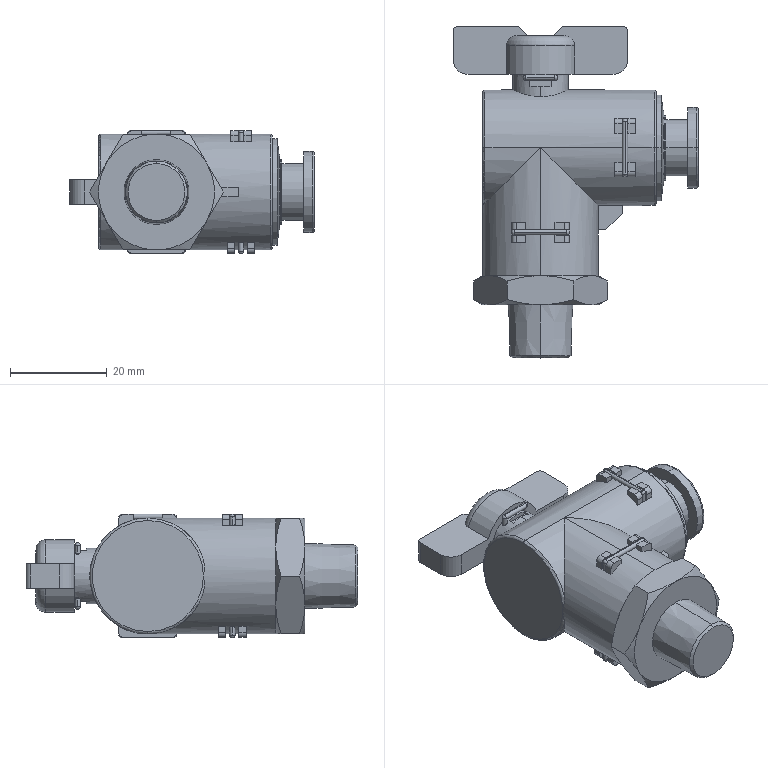Part | SolidWorks | features BaseBody 2 | 2 solids | 242 faces | box 50.7 x 68.7 x 25.6 mm | volume 31138 mm3 | plane 109 | cylinder 83 | cone 28 | sphere 12 | torus 10 | commonest cylinder face diameters 1.1 x36 2 x18 24 x6 4.6 x4 13.44 x4 15 x3